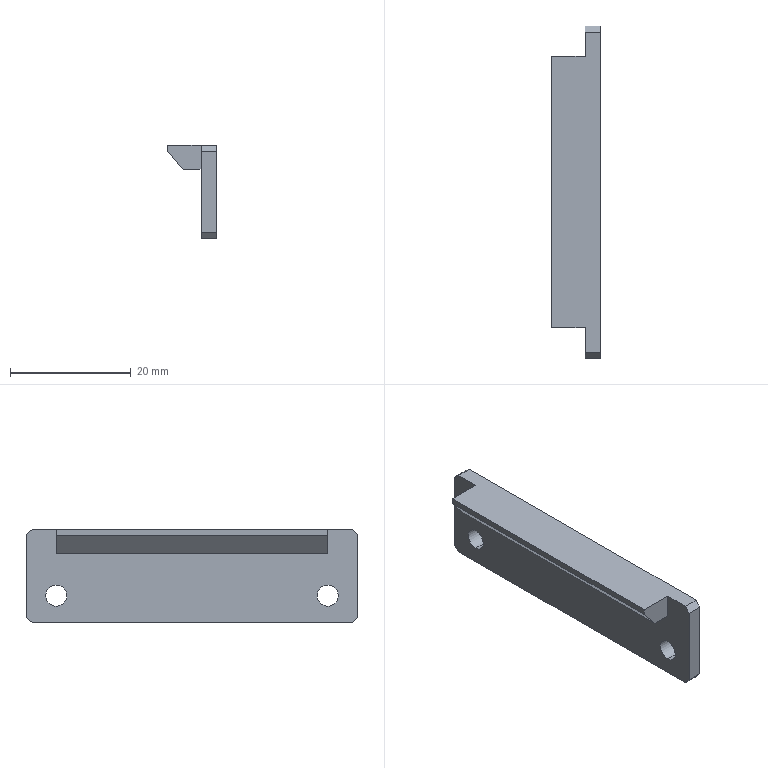Part | SolidWorks | features ICE 3, Chamfer 2, Extrusion 1 | 1 solid | 19 faces | box 8 x 55 x 15.5 mm | volume 2899 mm3 | plane 15 | cylinder 4 | commonest cylinder face diameters 3.5 x4
STEP:
#1=CARTESIAN_POINT('',(5.5,5.,-9.25));
#2=VERTEX_POINT('',#1);
#3=CARTESIAN_POINT('',(5.5,5.,-12.75));
#4=VERTEX_POINT('',#3);
#5=CARTESIAN_POINT('',(5.5,5.,-11.));
#6=DIRECTION('',(1.,0.,0.));
#7=DIRECTION('',(0.,0.,-1.));
#8=AXIS2_PLACEMENT_3D('',#5,#6,#7);
#9=CIRCLE('',#8,1.75);
#10=EDGE_CURVE('',#2,#4,#9,.T.);
#11=ORIENTED_EDGE('',*,*,#10,.F.);
#12=CARTESIAN_POINT('',(8.,5.,-9.25));
#13=VERTEX_POINT('',#12);
#14=CARTESIAN_POINT('',(-40.,5.,-9.25));
#15=DIRECTION('',(1.,0.,0.));
#16=VECTOR('',#15,1000.);
#17=LINE('',#14,#16);
#18=EDGE_CURVE('',#2,#13,#17,.T.);
#19=ORIENTED_EDGE('',*,*,#18,.T.);
#20=CARTESIAN_POINT('',(8.,5.,-12.75));
#21=VERTEX_POINT('',#20);
#22=CARTESIAN_POINT('',(8.,5.,-11.));
#23=DIRECTION('',(1.,0.,0.));
#24=DIRECTION('',(0.,0.,1.));
#25=AXIS2_PLACEMENT_3D('',#22,#23,#24);
#26=CIRCLE('',#25,1.75);
#27=EDGE_CURVE('',#13,#21,#26,.T.);
#28=ORIENTED_EDGE('',*,*,#27,.T.);
#29=CARTESIAN_POINT('',(-40.,5.,-12.75));
#30=DIRECTION('',(1.,0.,0.));
#31=VECTOR('',#30,1000.);
#32=LINE('',#29,#31);
#33=EDGE_CURVE('',#4,#21,#32,.T.);
#34=ORIENTED_EDGE('',*,*,#33,.F.);
#35=EDGE_LOOP('',(#11,#19,#28,#34));
#36=FACE_OUTER_BOUND('',#35,.T.);
#37=CARTESIAN_POINT('',(-40.,5.,-11.));
#38=DIRECTION('',(1.,0.,0.));
#39=DIRECTION('',(0.,0.,-1.));
#40=AXIS2_PLACEMENT_3D('',#37,#38,#39);
#41=CYLINDRICAL_SURFACE('',#40,1.75);
#42=ADVANCED_FACE('',(#36),#41,.F.);
#43=CARTESIAN_POINT('',(5.5,50.,-9.25));
#44=VERTEX_POINT('',#43);
#45=CARTESIAN_POINT('',(5.5,50.,-12.75));
#46=VERTEX_POINT('',#45);
#47=CARTESIAN_POINT('',(5.5,50.,-11.));
#48=DIRECTION('',(1.,0.,0.));
#49=DIRECTION('',(0.,0.,-1.));
#50=AXIS2_PLACEMENT_3D('',#47,#48,#49);
#51=CIRCLE('',#50,1.75);
#52=EDGE_CURVE('',#44,#46,#51,.T.);
#53=ORIENTED_EDGE('',*,*,#52,.F.);
#54=CARTESIAN_POINT('',(8.,50.,-9.25));
#55=VERTEX_POINT('',#54);
#56=CARTESIAN_POINT('',(-40.,50.,-9.25));
#57=DIRECTION('',(1.,0.,0.));
#58=VECTOR('',#57,1000.);
#59=LINE('',#56,#58);
#60=EDGE_CURVE('',#44,#55,#59,.T.);
#61=ORIENTED_EDGE('',*,*,#60,.T.);
#62=CARTESIAN_POINT('',(8.,50.,-12.75));
#63=VERTEX_POINT('',#62);
#64=CARTESIAN_POINT('',(8.,50.,-11.));
#65=DIRECTION('',(1.,0.,0.));
#66=DIRECTION('',(0.,0.,-1.));
#67=AXIS2_PLACEMENT_3D('',#64,#65,#66);
#68=CIRCLE('',#67,1.75);
#69=EDGE_CURVE('',#55,#63,#68,.T.);
#70=ORIENTED_EDGE('',*,*,#69,.T.);
#71=CARTESIAN_POINT('',(-40.,50.,-12.75));
#72=DIRECTION('',(1.,0.,0.));
#73=VECTOR('',#72,1000.);
#74=LINE('',#71,#73);
#75=EDGE_CURVE('',#46,#63,#74,.T.);
#76=ORIENTED_EDGE('',*,*,#75,.F.);
#77=EDGE_LOOP('',(#53,#61,#70,#76));
#78=FACE_OUTER_BOUND('',#77,.T.);
#79=CARTESIAN_POINT('',(-40.,50.,-11.));
#80=DIRECTION('',(1.,0.,0.));
#81=DIRECTION('',(0.,0.,-1.));
#82=AXIS2_PLACEMENT_3D('',#79,#80,#81);
#83=CYLINDRICAL_SURFACE('',#82,1.75);
#84=ADVANCED_FACE('',(#78),#83,.F.);
#85=CARTESIAN_POINT('',(0.,50.,-1.));
#86=VERTEX_POINT('',#85);
#87=CARTESIAN_POINT('',(0.,5.,-1.));
#88=VERTEX_POINT('',#87);
#89=CARTESIAN_POINT('',(0.,55.,-1.));
#90=DIRECTION('',(0.,-1.,0.));
#91=VECTOR('',#90,1000.);
#92=LINE('',#89,#91);
#93=EDGE_CURVE('',#86,#88,#92,.T.);
#94=ORIENTED_EDGE('',*,*,#93,.T.);
#95=CARTESIAN_POINT('',(0.,5.,0.));
#96=VERTEX_POINT('',#95);
#97=CARTESIAN_POINT('',(0.,5.,0.));
#98=DIRECTION('',(0.,0.,-1.));
#99=VECTOR('',#98,1000.);
#100=LINE('',#97,#99);
#101=EDGE_CURVE('',#96,#88,#100,.T.);
#102=ORIENTED_EDGE('',*,*,#101,.F.);
#103=CARTESIAN_POINT('',(0.,50.,0.));
#104=VERTEX_POINT('',#103);
#105=CARTESIAN_POINT('',(0.,55.,0.));
#106=DIRECTION('',(0.,-1.,0.));
#107=VECTOR('',#106,1000.);
#108=LINE('',#105,#107);
#109=EDGE_CURVE('',#104,#96,#108,.T.);
#110=ORIENTED_EDGE('',*,*,#109,.F.);
#111=CARTESIAN_POINT('',(0.,50.,0.));
#112=DIRECTION('',(0.,0.,-1.));
#113=VECTOR('',#112,1000.);
#114=LINE('',#111,#113);
#115=EDGE_CURVE('',#104,#86,#114,.T.);
#116=ORIENTED_EDGE('',*,*,#115,.T.);
#117=EDGE_LOOP('',(#94,#102,#110,#116));
#118=FACE_OUTER_BOUND('',#117,.T.);
#119=CARTESIAN_POINT('',(0.,55.,0.));
#120=DIRECTION('',(1.,0.,0.));
#121=DIRECTION('',(0.,0.,-1.));
#122=AXIS2_PLACEMENT_3D('',#119,#120,#121);
#123=PLANE('',#122);
#124=ADVANCED_FACE('',(#118),#123,.F.);
#125=CARTESIAN_POINT('',(5.5,5.,0.));
#126=VERTEX_POINT('',#125);
#127=CARTESIAN_POINT('',(5.5,0.8391,0.));
#128=VERTEX_POINT('',#127);
#129=CARTESIAN_POINT('',(5.5,0.,0.));
#130=DIRECTION('',(0.,-1.,0.));
#131=VECTOR('',#130,1000.);
#132=LINE('',#129,#131);
#133=EDGE_CURVE('',#126,#128,#132,.T.);
#134=ORIENTED_EDGE('',*,*,#133,.T.);
#135=CARTESIAN_POINT('',(8.,0.8391,0.));
#136=VERTEX_POINT('',#135);
#137=CARTESIAN_POINT('',(8.,0.8391,0.));
#138=DIRECTION('',(1.,0.,0.));
#139=VECTOR('',#138,1000.);
#140=LINE('',#137,#139);
#141=EDGE_CURVE('',#128,#136,#140,.T.);
#142=ORIENTED_EDGE('',*,*,#141,.T.);
#143=CARTESIAN_POINT('',(8.,54.,0.));
#144=VERTEX_POINT('',#143);
#145=CARTESIAN_POINT('',(8.,55.,0.));
#146=DIRECTION('',(0.,-1.,0.));
#147=VECTOR('',#146,1000.);
#148=LINE('',#145,#147);
#149=EDGE_CURVE('',#144,#136,#148,.T.);
#150=ORIENTED_EDGE('',*,*,#149,.F.);
#151=CARTESIAN_POINT('',(5.5,54.,0.));
#152=VERTEX_POINT('',#151);
#153=CARTESIAN_POINT('',(0.,54.,0.));
#154=DIRECTION('',(-1.,0.,0.));
#155=VECTOR('',#154,1000.);
#156=LINE('',#153,#155);
#157=EDGE_CURVE('',#144,#152,#156,.T.);
#158=ORIENTED_EDGE('',*,*,#157,.T.);
#159=CARTESIAN_POINT('',(5.5,50.,0.));
#160=VERTEX_POINT('',#159);
#161=CARTESIAN_POINT('',(5.5,55.,0.));
#162=DIRECTION('',(0.,-1.,0.));
#163=VECTOR('',#162,1000.);
#164=LINE('',#161,#163);
#165=EDGE_CURVE('',#152,#160,#164,.T.);
#166=ORIENTED_EDGE('',*,*,#165,.T.);
#167=CARTESIAN_POINT('',(0.,50.,0.));
#168=DIRECTION('',(-1.,0.,0.));
#169=VECTOR('',#168,1000.);
#170=LINE('',#167,#169);
#171=EDGE_CURVE('',#160,#104,#170,.T.);
#172=ORIENTED_EDGE('',*,*,#171,.T.);
#173=ORIENTED_EDGE('',*,*,#109,.T.);
#174=CARTESIAN_POINT('',(0.,5.,0.));
#175=DIRECTION('',(1.,0.,0.));
#176=VECTOR('',#175,1000.);
#177=LINE('',#174,#176);
#178=EDGE_CURVE('',#96,#126,#177,.T.);
#179=ORIENTED_EDGE('',*,*,#178,.T.);
#180=EDGE_LOOP('',(#134,#142,#150,#158,#166,#172,#173,#179));
#181=FACE_OUTER_BOUND('',#180,.T.);
#182=CARTESIAN_POINT('',(0.,55.,0.));
#183=DIRECTION('',(0.,0.,-1.));
#184=DIRECTION('',(-1.,0.,0.));
#185=AXIS2_PLACEMENT_3D('',#182,#183,#184);
#186=PLANE('',#185);
#187=ADVANCED_FACE('',(#181),#186,.F.);
#188=CARTESIAN_POINT('',(8.,5.,-11.));
#189=DIRECTION('',(1.,0.,0.));
#190=DIRECTION('',(0.,0.,1.));
#191=AXIS2_PLACEMENT_3D('',#188,#189,#190);
#192=CIRCLE('',#191,1.75);
#193=EDGE_CURVE('',#21,#13,#192,.T.);
#194=ORIENTED_EDGE('',*,*,#193,.F.);
#195=ORIENTED_EDGE('',*,*,#27,.F.);
#196=EDGE_LOOP('',(#194,#195));
#197=FACE_BOUND('',#196,.T.);
#198=CARTESIAN_POINT('',(8.,50.,-11.));
#199=DIRECTION('',(1.,0.,0.));
#200=DIRECTION('',(0.,0.,-1.));
#201=AXIS2_PLACEMENT_3D('',#198,#199,#200);
#202=CIRCLE('',#201,1.75);
#203=EDGE_CURVE('',#63,#55,#202,.T.);
#204=ORIENTED_EDGE('',*,*,#203,.F.);
#205=ORIENTED_EDGE('',*,*,#69,.F.);
#206=EDGE_LOOP('',(#204,#205));
#207=FACE_BOUND('',#206,.T.);
#208=ORIENTED_EDGE('',*,*,#149,.T.);
#209=CARTESIAN_POINT('',(8.,0.,-1.));
#210=VERTEX_POINT('',#209);
#211=CARTESIAN_POINT('',(8.,0.8391,0.));
#212=DIRECTION('',(0.,-0.6428,-0.766));
#213=VECTOR('',#212,1000.);
#214=LINE('',#211,#213);
#215=EDGE_CURVE('',#136,#210,#214,.T.);
#216=ORIENTED_EDGE('',*,*,#215,.T.);
#217=CARTESIAN_POINT('',(8.,0.,-14.5));
#218=VERTEX_POINT('',#217);
#219=CARTESIAN_POINT('',(8.,0.,0.));
#220=DIRECTION('',(0.,0.,-1.));
#221=VECTOR('',#220,1000.);
#222=LINE('',#219,#221);
#223=EDGE_CURVE('',#210,#218,#222,.T.);
#224=ORIENTED_EDGE('',*,*,#223,.T.);
#225=CARTESIAN_POINT('',(8.,0.8391,-15.5));
#226=VERTEX_POINT('',#225);
#227=CARTESIAN_POINT('',(8.,0.8391,-15.5));
#228=DIRECTION('',(0.,0.6428,-0.766));
#229=VECTOR('',#228,1000.);
#230=LINE('',#227,#229);
#231=EDGE_CURVE('',#218,#226,#230,.T.);
#232=ORIENTED_EDGE('',*,*,#231,.T.);
#233=CARTESIAN_POINT('',(8.,54.,-15.5));
#234=VERTEX_POINT('',#233);
#235=CARTESIAN_POINT('',(8.,55.,-15.5));
#236=DIRECTION('',(0.,-1.,0.));
#237=VECTOR('',#236,1000.);
#238=LINE('',#235,#237);
#239=EDGE_CURVE('',#234,#226,#238,.T.);
#240=ORIENTED_EDGE('',*,*,#239,.F.);
#241=CARTESIAN_POINT('',(8.,55.,-14.661));
#242=VERTEX_POINT('',#241);
#243=CARTESIAN_POINT('',(8.,55.,-14.661));
#244=DIRECTION('',(0.,0.766,0.6428));
#245=VECTOR('',#244,1000.);
#246=LINE('',#243,#245);
#247=EDGE_CURVE('',#234,#242,#246,.T.);
#248=ORIENTED_EDGE('',*,*,#247,.T.);
#249=CARTESIAN_POINT('',(8.,55.,-0.8391));
#250=VERTEX_POINT('',#249);
#251=CARTESIAN_POINT('',(8.,55.,0.));
#252=DIRECTION('',(0.,0.,-1.));
#253=VECTOR('',#252,1000.);
#254=LINE('',#251,#253);
#255=EDGE_CURVE('',#250,#242,#254,.T.);
#256=ORIENTED_EDGE('',*,*,#255,.F.);
#257=CARTESIAN_POINT('',(8.,55.,-0.8391));
#258=DIRECTION('',(0.,-0.766,0.6428));
#259=VECTOR('',#258,1000.);
#260=LINE('',#257,#259);
#261=EDGE_CURVE('',#250,#144,#260,.T.);
#262=ORIENTED_EDGE('',*,*,#261,.T.);
#263=EDGE_LOOP('',(#208,#216,#224,#232,#240,#248,#256,#262));
#264=FACE_OUTER_BOUND('',#263,.T.);
#265=CARTESIAN_POINT('',(8.,55.,0.));
#266=DIRECTION('',(-1.,0.,0.));
#267=DIRECTION('',(0.,0.,1.));
#268=AXIS2_PLACEMENT_3D('',#265,#266,#267);
#269=PLANE('',#268);
#270=ADVANCED_FACE('',(#197,#207,#264),#269,.F.);
#271=ORIENTED_EDGE('',*,*,#239,.T.);
#272=CARTESIAN_POINT('',(5.5,0.8391,-15.5));
#273=VERTEX_POINT('',#272);
#274=CARTESIAN_POINT('',(5.5,0.8391,-15.5));
#275=DIRECTION('',(-1.,0.,0.));
#276=VECTOR('',#275,1000.);
#277=LINE('',#274,#276);
#278=EDGE_CURVE('',#226,#273,#277,.T.);
#279=ORIENTED_EDGE('',*,*,#278,.T.);
#280=CARTESIAN_POINT('',(5.5,54.,-15.5));
#281=VERTEX_POINT('',#280);
#282=CARTESIAN_POINT('',(5.5,0.,-15.5));
#283=DIRECTION('',(0.,1.,0.));
#284=VECTOR('',#283,1000.);
#285=LINE('',#282,#284);
#286=EDGE_CURVE('',#273,#281,#285,.T.);
#287=ORIENTED_EDGE('',*,*,#286,.T.);
#288=CARTESIAN_POINT('',(0.,54.,-15.5));
#289=DIRECTION('',(1.,0.,0.));
#290=VECTOR('',#289,1000.);
#291=LINE('',#288,#290);
#292=EDGE_CURVE('',#281,#234,#291,.T.);
#293=ORIENTED_EDGE('',*,*,#292,.T.);
#294=EDGE_LOOP('',(#271,#279,#287,#293));
#295=FACE_OUTER_BOUND('',#294,.T.);
#296=CARTESIAN_POINT('',(0.,55.,-15.5));
#297=DIRECTION('',(0.,0.,1.));
#298=DIRECTION('',(1.,0.,0.));
#299=AXIS2_PLACEMENT_3D('',#296,#297,#298);
#300=PLANE('',#299);
#301=ADVANCED_FACE('',(#295),#300,.F.);
#302=CARTESIAN_POINT('',(5.5,55.,-0.8391));
#303=VERTEX_POINT('',#302);
#304=CARTESIAN_POINT('',(5.5,55.,-14.661));
#305=VERTEX_POINT('',#304);
#306=CARTESIAN_POINT('',(5.5,55.,-15.5));
#307=DIRECTION('',(0.,0.,-1.));
#308=VECTOR('',#307,1000.);
#309=LINE('',#306,#308);
#310=EDGE_CURVE('',#303,#305,#309,.T.);
#311=ORIENTED_EDGE('',*,*,#310,.F.);
#312=CARTESIAN_POINT('',(0.,55.,-0.8391));
#313=DIRECTION('',(1.,0.,0.));
#314=VECTOR('',#313,1000.);
#315=LINE('',#312,#314);
#316=EDGE_CURVE('',#303,#250,#315,.T.);
#317=ORIENTED_EDGE('',*,*,#316,.T.);
#318=ORIENTED_EDGE('',*,*,#255,.T.);
#319=CARTESIAN_POINT('',(0.,55.,-14.661));
#320=DIRECTION('',(-1.,0.,0.));
#321=VECTOR('',#320,1000.);
#322=LINE('',#319,#321);
#323=EDGE_CURVE('',#242,#305,#322,.T.);
#324=ORIENTED_EDGE('',*,*,#323,.T.);
#325=EDGE_LOOP('',(#311,#317,#318,#324));
#326=FACE_OUTER_BOUND('',#325,.T.);
#327=CARTESIAN_POINT('',(0.,55.,0.));
#328=DIRECTION('',(0.,-1.,0.));
#329=DIRECTION('',(0.,0.,-1.));
#330=AXIS2_PLACEMENT_3D('',#327,#328,#329);
#331=PLANE('',#330);
#332=ADVANCED_FACE('',(#326),#331,.F.);
#333=ORIENTED_EDGE('',*,*,#223,.F.);
#334=CARTESIAN_POINT('',(5.5,0.,-1.));
#335=VERTEX_POINT('',#334);
#336=CARTESIAN_POINT('',(5.5,0.,-1.));
#337=DIRECTION('',(-1.,0.,0.));
#338=VECTOR('',#337,1000.);
#339=LINE('',#336,#338);
#340=EDGE_CURVE('',#210,#335,#339,.T.);
#341=ORIENTED_EDGE('',*,*,#340,.T.);
#342=CARTESIAN_POINT('',(5.5,0.,-14.5));
#343=VERTEX_POINT('',#342);
#344=CARTESIAN_POINT('',(5.5,0.,-15.5));
#345=DIRECTION('',(0.,0.,-1.));
#346=VECTOR('',#345,1000.);
#347=LINE('',#344,#346);
#348=EDGE_CURVE('',#335,#343,#347,.T.);
#349=ORIENTED_EDGE('',*,*,#348,.T.);
#350=CARTESIAN_POINT('',(8.,0.,-14.5));
#351=DIRECTION('',(1.,0.,0.));
#352=VECTOR('',#351,1000.);
#353=LINE('',#350,#352);
#354=EDGE_CURVE('',#343,#218,#353,.T.);
#355=ORIENTED_EDGE('',*,*,#354,.T.);
#356=EDGE_LOOP('',(#333,#341,#349,#355));
#357=FACE_OUTER_BOUND('',#356,.T.);
#358=CARTESIAN_POINT('',(0.,0.,0.));
#359=DIRECTION('',(0.,-1.,0.));
#360=DIRECTION('',(0.,0.,-1.));
#361=AXIS2_PLACEMENT_3D('',#358,#359,#360);
#362=PLANE('',#361);
#363=ADVANCED_FACE('',(#357),#362,.T.);
#364=CARTESIAN_POINT('',(5.5,5.,-11.));
#365=DIRECTION('',(1.,0.,0.));
#366=DIRECTION('',(0.,0.,-1.));
#367=AXIS2_PLACEMENT_3D('',#364,#365,#366);
#368=CIRCLE('',#367,1.75);
#369=EDGE_CURVE('',#4,#2,#368,.T.);
#370=ORIENTED_EDGE('',*,*,#369,.T.);
#371=ORIENTED_EDGE('',*,*,#10,.T.);
#372=EDGE_LOOP('',(#370,#371));
#373=FACE_BOUND('',#372,.T.);
#374=CARTESIAN_POINT('',(5.5,50.,-11.));
#375=DIRECTION('',(1.,0.,0.));
#376=DIRECTION('',(0.,0.,-1.));
#377=AXIS2_PLACEMENT_3D('',#374,#375,#376);
#378=CIRCLE('',#377,1.75);
#379=EDGE_CURVE('',#46,#44,#378,.T.);
#380=ORIENTED_EDGE('',*,*,#379,.T.);
#381=ORIENTED_EDGE('',*,*,#52,.T.);
#382=EDGE_LOOP('',(#380,#381));
#383=FACE_BOUND('',#382,.T.);
#384=ORIENTED_EDGE('',*,*,#348,.F.);
#385=CARTESIAN_POINT('',(5.5,0.8391,0.));
#386=DIRECTION('',(0.,0.6428,0.766));
#387=VECTOR('',#386,1000.);
#388=LINE('',#385,#387);
#389=EDGE_CURVE('',#335,#128,#388,.T.);
#390=ORIENTED_EDGE('',*,*,#389,.T.);
#391=ORIENTED_EDGE('',*,*,#133,.F.);
#392=CARTESIAN_POINT('',(5.5,5.,-4.));
#393=VERTEX_POINT('',#392);
#394=CARTESIAN_POINT('',(5.5,5.,0.));
#395=DIRECTION('',(0.,0.,-1.));
#396=VECTOR('',#395,1000.);
#397=LINE('',#394,#396);
#398=EDGE_CURVE('',#126,#393,#397,.T.);
#399=ORIENTED_EDGE('',*,*,#398,.T.);
#400=CARTESIAN_POINT('',(5.5,50.,-4.));
#401=VERTEX_POINT('',#400);
#402=CARTESIAN_POINT('',(5.5,0.,-4.));
#403=DIRECTION('',(0.,1.,0.));
#404=VECTOR('',#403,1000.);
#405=LINE('',#402,#404);
#406=EDGE_CURVE('',#393,#401,#405,.T.);
#407=ORIENTED_EDGE('',*,*,#406,.T.);
#408=CARTESIAN_POINT('',(5.5,50.,0.));
#409=DIRECTION('',(0.,0.,-1.));
#410=VECTOR('',#409,1000.);
#411=LINE('',#408,#410);
#412=EDGE_CURVE('',#160,#401,#411,.T.);
#413=ORIENTED_EDGE('',*,*,#412,.F.);
#414=ORIENTED_EDGE('',*,*,#165,.F.);
#415=CARTESIAN_POINT('',(5.5,55.,-0.8391));
#416=DIRECTION('',(0.,0.766,-0.6428));
#417=VECTOR('',#416,1000.);
#418=LINE('',#415,#417);
#419=EDGE_CURVE('',#152,#303,#418,.T.);
#420=ORIENTED_EDGE('',*,*,#419,.T.);
#421=ORIENTED_EDGE('',*,*,#310,.T.);
#422=CARTESIAN_POINT('',(5.5,55.,-14.661));
#423=DIRECTION('',(0.,-0.766,-0.6428));
#424=VECTOR('',#423,1000.);
#425=LINE('',#422,#424);
#426=EDGE_CURVE('',#305,#281,#425,.T.);
#427=ORIENTED_EDGE('',*,*,#426,.T.);
#428=ORIENTED_EDGE('',*,*,#286,.F.);
#429=CARTESIAN_POINT('',(5.5,0.8391,-15.5));
#430=DIRECTION('',(0.,-0.6428,0.766));
#431=VECTOR('',#430,1000.);
#432=LINE('',#429,#431);
#433=EDGE_CURVE('',#273,#343,#432,.T.);
#434=ORIENTED_EDGE('',*,*,#433,.T.);
#435=EDGE_LOOP('',(#384,#390,#391,#399,#407,#413,#414,#420,#421,#427,#428,#434));
#436=FACE_OUTER_BOUND('',#435,.T.);
#437=CARTESIAN_POINT('',(5.5,0.,-15.5));
#438=DIRECTION('',(1.,0.,0.));
#439=DIRECTION('',(0.,0.,-1.));
#440=AXIS2_PLACEMENT_3D('',#437,#438,#439);
#441=PLANE('',#440);
#442=ADVANCED_FACE('',(#373,#383,#436),#441,.F.);
#443=ORIENTED_EDGE('',*,*,#406,.F.);
#444=CARTESIAN_POINT('',(2.517,5.,-4.));
#445=VERTEX_POINT('',#444);
#446=CARTESIAN_POINT('',(0.,5.,-4.));
#447=DIRECTION('',(1.,0.,0.));
#448=VECTOR('',#447,1000.);
#449=LINE('',#446,#448);
#450=EDGE_CURVE('',#445,#393,#449,.T.);
#451=ORIENTED_EDGE('',*,*,#450,.F.);
#452=CARTESIAN_POINT('',(2.517,50.,-4.));
#453=VERTEX_POINT('',#452);
#454=CARTESIAN_POINT('',(2.517,0.,-4.));
#455=DIRECTION('',(0.,1.,0.));
#456=VECTOR('',#455,1000.);
#457=LINE('',#454,#456);
#458=EDGE_CURVE('',#445,#453,#457,.T.);
#459=ORIENTED_EDGE('',*,*,#458,.T.);
#460=CARTESIAN_POINT('',(0.,50.,-4.));
#461=DIRECTION('',(-1.,0.,0.));
#462=VECTOR('',#461,1000.);
#463=LINE('',#460,#462);
#464=EDGE_CURVE('',#401,#453,#463,.T.);
#465=ORIENTED_EDGE('',*,*,#464,.F.);
#466=EDGE_LOOP('',(#443,#451,#459,#465));
#467=FACE_OUTER_BOUND('',#466,.T.);
#468=CARTESIAN_POINT('',(0.,0.,-4.));
#469=DIRECTION('',(0.,0.,1.));
#470=DIRECTION('',(1.,0.,0.));
#471=AXIS2_PLACEMENT_3D('',#468,#469,#470);
#472=PLANE('',#471);
#473=ADVANCED_FACE('',(#467),#472,.F.);
#474=CARTESIAN_POINT('',(2.517,5.,-4.));
#475=DIRECTION('',(0.6428,0.,-0.766));
#476=VECTOR('',#475,1000.);
#477=LINE('',#474,#476);
#478=EDGE_CURVE('',#88,#445,#477,.T.);
#479=ORIENTED_EDGE('',*,*,#478,.F.);
#480=ORIENTED_EDGE('',*,*,#93,.F.);
#481=CARTESIAN_POINT('',(2.517,50.,-4.));
#482=DIRECTION('',(-0.6428,0.,0.766));
#483=VECTOR('',#482,1000.);
#484=LINE('',#481,#483);
#485=EDGE_CURVE('',#453,#86,#484,.T.);
#486=ORIENTED_EDGE('',*,*,#485,.F.);
#487=ORIENTED_EDGE('',*,*,#458,.F.);
#488=EDGE_LOOP('',(#479,#480,#486,#487));
#489=FACE_OUTER_BOUND('',#488,.T.);
#490=CARTESIAN_POINT('',(2.517,0.,-4.));
#491=DIRECTION('',(0.766,0.,0.6428));
#492=DIRECTION('',(0.,1.,0.));
#493=AXIS2_PLACEMENT_3D('',#490,#491,#492);
#494=PLANE('',#493);
#495=ADVANCED_FACE('',(#489),#494,.F.);
#496=ORIENTED_EDGE('',*,*,#60,.F.);
#497=ORIENTED_EDGE('',*,*,#379,.F.);
#498=ORIENTED_EDGE('',*,*,#75,.T.);
#499=ORIENTED_EDGE('',*,*,#203,.T.);
#500=EDGE_LOOP('',(#496,#497,#498,#499));
#501=FACE_OUTER_BOUND('',#500,.T.);
#502=CARTESIAN_POINT('',(-40.,50.,-11.));
#503=DIRECTION('',(1.,0.,0.));
#504=DIRECTION('',(0.,0.,-1.));
#505=AXIS2_PLACEMENT_3D('',#502,#503,#504);
#506=CYLINDRICAL_SURFACE('',#505,1.75);
#507=ADVANCED_FACE('',(#501),#506,.F.);
#508=ORIENTED_EDGE('',*,*,#18,.F.);
#509=ORIENTED_EDGE('',*,*,#369,.F.);
#510=ORIENTED_EDGE('',*,*,#33,.T.);
#511=ORIENTED_EDGE('',*,*,#193,.T.);
#512=EDGE_LOOP('',(#508,#509,#510,#511));
#513=FACE_OUTER_BOUND('',#512,.T.);
#514=CARTESIAN_POINT('',(-40.,5.,-11.));
#515=DIRECTION('',(1.,0.,0.));
#516=DIRECTION('',(0.,0.,-1.));
#517=AXIS2_PLACEMENT_3D('',#514,#515,#516);
#518=CYLINDRICAL_SURFACE('',#517,1.75);
#519=ADVANCED_FACE('',(#513),#518,.F.);
#520=ORIENTED_EDGE('',*,*,#485,.T.);
#521=ORIENTED_EDGE('',*,*,#115,.F.);
#522=ORIENTED_EDGE('',*,*,#171,.F.);
#523=ORIENTED_EDGE('',*,*,#412,.T.);
#524=ORIENTED_EDGE('',*,*,#464,.T.);
#525=EDGE_LOOP('',(#520,#521,#522,#523,#524));
#526=FACE_OUTER_BOUND('',#525,.T.);
#527=CARTESIAN_POINT('',(0.,50.,0.));
#528=DIRECTION('',(0.,-1.,0.));
#529=DIRECTION('',(0.,0.,-1.));
#530=AXIS2_PLACEMENT_3D('',#527,#528,#529);
#531=PLANE('',#530);
#532=ADVANCED_FACE('',(#526),#531,.F.);
#533=ORIENTED_EDGE('',*,*,#478,.T.);
#534=ORIENTED_EDGE('',*,*,#450,.T.);
#535=ORIENTED_EDGE('',*,*,#398,.F.);
#536=ORIENTED_EDGE('',*,*,#178,.F.);
#537=ORIENTED_EDGE('',*,*,#101,.T.);
#538=EDGE_LOOP('',(#533,#534,#535,#536,#537));
#539=FACE_OUTER_BOUND('',#538,.T.);
#540=CARTESIAN_POINT('',(0.,5.,0.));
#541=DIRECTION('',(0.,1.,0.));
#542=DIRECTION('',(-1.,0.,0.));
#543=AXIS2_PLACEMENT_3D('',#540,#541,#542);
#544=PLANE('',#543);
#545=ADVANCED_FACE('',(#539),#544,.F.);
#546=ORIENTED_EDGE('',*,*,#389,.F.);
#547=ORIENTED_EDGE('',*,*,#340,.F.);
#548=ORIENTED_EDGE('',*,*,#215,.F.);
#549=ORIENTED_EDGE('',*,*,#141,.F.);
#550=EDGE_LOOP('',(#546,#547,#548,#549));
#551=FACE_OUTER_BOUND('',#550,.T.);
#552=CARTESIAN_POINT('',(0.,0.8391,0.));
#553=DIRECTION('',(0.,-0.766,0.6428));
#554=DIRECTION('',(-1.,0.,0.));
#555=AXIS2_PLACEMENT_3D('',#552,#553,#554);
#556=PLANE('',#555);
#557=ADVANCED_FACE('',(#551),#556,.T.);
#558=ORIENTED_EDGE('',*,*,#419,.F.);
#559=ORIENTED_EDGE('',*,*,#157,.F.);
#560=ORIENTED_EDGE('',*,*,#261,.F.);
#561=ORIENTED_EDGE('',*,*,#316,.F.);
#562=EDGE_LOOP('',(#558,#559,#560,#561));
#563=FACE_OUTER_BOUND('',#562,.T.);
#564=CARTESIAN_POINT('',(0.,55.,-0.8391));
#565=DIRECTION('',(0.,-0.6428,-0.766));
#566=DIRECTION('',(1.,0.,0.));
#567=AXIS2_PLACEMENT_3D('',#564,#565,#566);
#568=PLANE('',#567);
#569=ADVANCED_FACE('',(#563),#568,.F.);
#570=ORIENTED_EDGE('',*,*,#231,.F.);
#571=ORIENTED_EDGE('',*,*,#354,.F.);
#572=ORIENTED_EDGE('',*,*,#433,.F.);
#573=ORIENTED_EDGE('',*,*,#278,.F.);
#574=EDGE_LOOP('',(#570,#571,#572,#573));
#575=FACE_OUTER_BOUND('',#574,.T.);
#576=CARTESIAN_POINT('',(0.,0.8391,-15.5));
#577=DIRECTION('',(0.,-0.766,-0.6428));
#578=DIRECTION('',(1.,0.,0.));
#579=AXIS2_PLACEMENT_3D('',#576,#577,#578);
#580=PLANE('',#579);
#581=ADVANCED_FACE('',(#575),#580,.T.);
#582=ORIENTED_EDGE('',*,*,#247,.F.);
#583=ORIENTED_EDGE('',*,*,#292,.F.);
#584=ORIENTED_EDGE('',*,*,#426,.F.);
#585=ORIENTED_EDGE('',*,*,#323,.F.);
#586=EDGE_LOOP('',(#582,#583,#584,#585));
#587=FACE_OUTER_BOUND('',#586,.T.);
#588=CARTESIAN_POINT('',(0.,55.,-14.661));
#589=DIRECTION('',(0.,-0.6428,0.766));
#590=DIRECTION('',(-1.,0.,0.));
#591=AXIS2_PLACEMENT_3D('',#588,#589,#590);
#592=PLANE('',#591);
#593=ADVANCED_FACE('',(#587),#592,.F.);
#594=CLOSED_SHELL('',(#42,#84,#124,#187,#270,#301,#332,#363,#442,#473,#495,#507,#519,#532,#545,#557,#569,#581,#593));
#595=MANIFOLD_SOLID_BREP('',#594);
#596=CARTESIAN_POINT('',(0.,0.,0.));
#597=DIRECTION('',(0.,0.,1.));
#598=DIRECTION('',(1.,0.,0.));
#599=AXIS2_PLACEMENT_3D('',#596,#597,#598);
#600=(LENGTH_UNIT()NAMED_UNIT(*)SI_UNIT(.MILLI.,.METRE.));
#601=UNCERTAINTY_MEASURE_WITH_UNIT(LENGTH_MEASURE(0.00001),#600,'','');
#602=(NAMED_UNIT(*)PLANE_ANGLE_UNIT()SI_UNIT($,.RADIAN.));
#603=(NAMED_UNIT(*)SI_UNIT($,.STERADIAN.)SOLID_ANGLE_UNIT());
#604=(GEOMETRIC_REPRESENTATION_CONTEXT(3)GLOBAL_UNCERTAINTY_ASSIGNED_CONTEXT((#601))GLOBAL_UNIT_ASSIGNED_CONTEXT((#600,#602,#603))REPRESENTATION_CONTEXT('',''));
#605=ADVANCED_BREP_SHAPE_REPRESENTATION('',(#595,#599),#604);